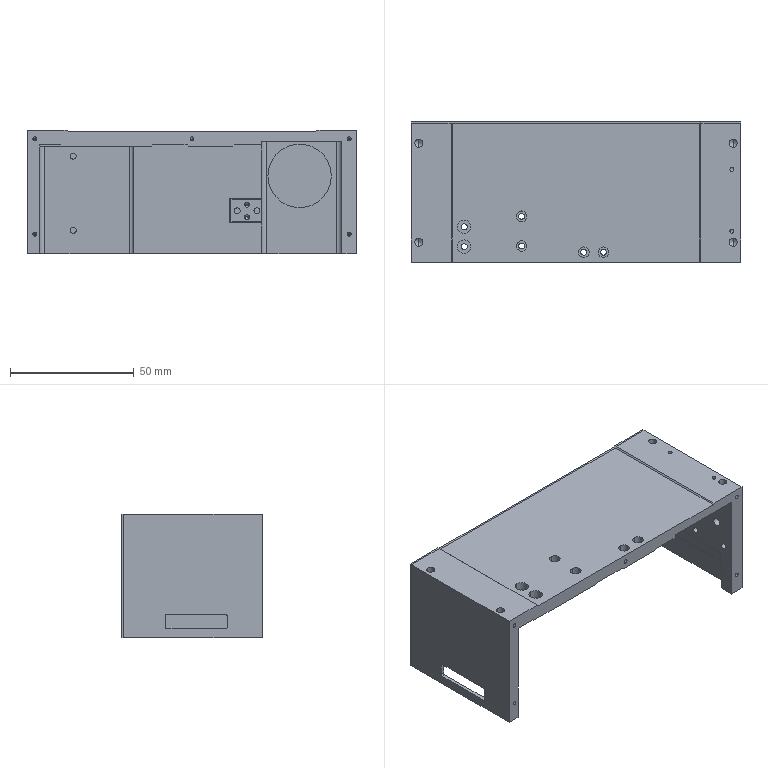NC program | NX | posted with a generic post | part box 133 x 56.74 x 50 mm
Whole program:
N10 G17 G21 G94 G90
(DRILLING_COPY_1 , TOOL : D6A45)
N12 T07 M6
N14 G54
N16 G17 G0 G90 X19.13 Y-28.5 B0. C0. S5000 M3
N18 G43 Z30. H7
N20 G94 G81 G98 Z-1. F250. R3.
N22 X13.13 Y-18.5
N24 X9.13 Y-8.5
N26 X5.13 Y-18.5
N28 X-0.87 Y-28.5
N30 X-7.87
N32 X-11.87 Y-18.5
N34 X-15.87 Y-8.5
N36 X-19.87 Y-18.5
N38 X-23.87 Y-28.5
N40 G80
N42 G0 X-23.87 Y-28.5 Z30.
N44 M5
(DRILLING_COPY_COPY_COPY_COPY , TOOL : 2.5ZT)
N46 T08 M6
N48 G54
N50 G17 G0 G90 X-15.87 Y-8.5 B0. C0. S2000 M3
N52 G43 Z30. H8
N54 G94 G83 G98 Z-8.251 F150. Q2. R3.
N56 X-23.87 Y-28.5
N58 X-7.87
N60 X9.13 Y-8.5
N62 X-0.87 Y-28.5
N64 X19.13
N66 G80
N68 G0 X19.13 Y-28.5 Z30.
N70 M5
(DRILLING_COPY_COPY_COPY_COPY_COPY , TOOL : 3.4ZT)
N72 T02 M6
N74 G54
N76 G17 G0 G90 X-19.87 Y-18.5 B0. C0. S2000 M3
N78 G43 Z30. H2
N80 G94 G83 G98 Z-8.521 F150. Q2. R-0.4
N82 X-11.87
N84 X5.13
N86 X13.13
N88 G80
N90 G0 X13.13 Y-18.5 Z30.
N92 M5
(HOLE_MILLING_COPY , TOOL : D4)
N94 T04 M6
N96 G54
N98 G17 G0 G90 X-19.87 Y-18.5 B0. C0. S9500 M3
N100 G43 Z30. H4
N102 Z0.5
N104 G94 G3 X-18.995 Y-19.375 R0.875 F1250.
N106 X-18.12 Y-18.5 R0.875
N108 X-18.12 Y-18.5 Z0.25 I-1.75 J0.
N110 X-18.12 Y-18.5 Z0. I-1.75 J0.
N112 X-18.12 Y-18.5 Z-0.25 I-1.75 J0.
N114 X-18.12 Y-18.5 Z-0.5 I-1.75 J0.
N116 X-18.12 Y-18.5 Z-0.75 I-1.75 J0.
N118 X-18.12 Y-18.5 Z-1. I-1.75 J0.
N120 X-18.12 Y-18.5 Z-1.25 I-1.75 J0.
N122 X-18.12 Y-18.5 Z-1.5 I-1.75 J0.
N124 X-18.12 Y-18.5 Z-1.75 I-1.75 J0.
N126 X-18.12 Y-18.5 Z-2. I-1.75 J0.
N128 X-18.12 Y-18.5 Z-2.25 I-1.75 J0.
N130 X-18.12 Y-18.5 Z-2.5 I-1.75 J0.
N132 X-18.12 Y-18.5 Z-2.75 I-1.75 J0.
N134 X-18.12 Y-18.5 Z-3. I-1.75 J0.
N136 X-18.12 Y-18.5 Z-3.25 I-1.75 J0.
N138 X-21.286 Y-19.529 Z-3.4 R-1.75
N140 X-18.841 Y-19.916 R1.75
N142 X-21.286 Y-19.529 R-1.75
N144 X-20.064 Y-19.722 R0.875
N146 X-19.87 Y-18.5 R0.875
N148 G0 Z30.
N150 X-11.87
N152 Z0.5
N154 G3 X-10.995 Y-19.375 R0.875
N156 X-10.12 Y-18.5 R0.875
N158 X-10.12 Y-18.5 Z0.25 I-1.75 J0.
N160 X-10.12 Y-18.5 Z0. I-1.75 J0.
N162 X-10.12 Y-18.5 Z-0.25 I-1.75 J0.
N164 X-10.12 Y-18.5 Z-0.5 I-1.75 J0.
N166 X-10.12 Y-18.5 Z-0.75 I-1.75 J0.
N168 X-10.12 Y-18.5 Z-1. I-1.75 J0.
N170 X-10.12 Y-18.5 Z-1.25 I-1.75 J0.
N172 X-10.12 Y-18.5 Z-1.5 I-1.75 J0.
N174 X-10.12 Y-18.5 Z-1.75 I-1.75 J0.
N176 X-10.12 Y-18.5 Z-2. I-1.75 J0.
N178 X-10.12 Y-18.5 Z-2.25 I-1.75 J0.
N180 X-10.12 Y-18.5 Z-2.5 I-1.75 J0.
N182 X-10.12 Y-18.5 Z-2.75 I-1.75 J0.
N184 X-10.12 Y-18.5 Z-3. I-1.75 J0.
N186 X-10.12 Y-18.5 Z-3.25 I-1.75 J0.
N188 X-13.286 Y-19.529 Z-3.4 R-1.75
N190 X-10.841 Y-19.916 R1.75
N192 X-13.286 Y-19.529 R-1.75
N194 X-12.064 Y-19.722 R0.875
N196 X-11.87 Y-18.5 R0.875
N198 G0 Z30.
N200 X5.13
N202 Z0.5
N204 G3 X6.005 Y-19.375 R0.875
N206 X6.88 Y-18.5 R0.875
N208 X6.88 Y-18.5 Z0.25 I-1.75 J0.
N210 X6.88 Y-18.5 Z0. I-1.75 J0.
N212 X6.88 Y-18.5 Z-0.25 I-1.75 J0.
N214 X6.88 Y-18.5 Z-0.5 I-1.75 J0.
N216 X6.88 Y-18.5 Z-0.75 I-1.75 J0.
N218 X6.88 Y-18.5 Z-1. I-1.75 J0.
N220 X6.88 Y-18.5 Z-1.25 I-1.75 J0.
N222 X6.88 Y-18.5 Z-1.5 I-1.75 J0.
N224 X6.88 Y-18.5 Z-1.75 I-1.75 J0.
N226 X6.88 Y-18.5 Z-2. I-1.75 J0.
N228 X6.88 Y-18.5 Z-2.25 I-1.75 J0.
N230 X6.88 Y-18.5 Z-2.5 I-1.75 J0.
N232 X6.88 Y-18.5 Z-2.75 I-1.75 J0.
N234 X6.88 Y-18.5 Z-3. I-1.75 J0.
N236 X6.88 Y-18.5 Z-3.25 I-1.75 J0.
N238 X3.714 Y-19.529 Z-3.4 R-1.75
N240 X6.159 Y-19.916 R1.75
N242 X3.714 Y-19.529 R-1.75
N244 X4.936 Y-19.722 R0.875
N246 X5.13 Y-18.5 R0.875
N248 G0 Z30.
N250 X13.13
N252 Z0.5
N254 G3 X14.005 Y-19.375 R0.875
N256 X14.88 Y-18.5 R0.875
N258 X14.88 Y-18.5 Z0.25 I-1.75 J0.
N260 X14.88 Y-18.5 Z0. I-1.75 J0.
N262 X14.88 Y-18.5 Z-0.25 I-1.75 J0.
N264 X14.88 Y-18.5 Z-0.5 I-1.75 J0.
N266 X14.88 Y-18.5 Z-0.75 I-1.75 J0.
N268 X14.88 Y-18.5 Z-1. I-1.75 J0.
N270 X14.88 Y-18.5 Z-1.25 I-1.75 J0.
N272 X14.88 Y-18.5 Z-1.5 I-1.75 J0.
N274 X14.88 Y-18.5 Z-1.75 I-1.75 J0.
N276 X14.88 Y-18.5 Z-2. I-1.75 J0.
N278 X14.88 Y-18.5 Z-2.25 I-1.75 J0.
N280 X14.88 Y-18.5 Z-2.5 I-1.75 J0.
N282 X14.88 Y-18.5 Z-2.75 I-1.75 J0.
N284 X14.88 Y-18.5 Z-3. I-1.75 J0.
N286 X14.88 Y-18.5 Z-3.25 I-1.75 J0.
N288 X11.714 Y-19.529 Z-3.4 R-1.75
N290 X14.159 Y-19.916 R1.75
N292 X11.714 Y-19.529 R-1.75
N294 X12.936 Y-19.722 R0.875
N296 X13.13 Y-18.5 R0.875
N298 G0 Z30.
N300 M5
(PLANAR_MILL_COPY_1_COPY_COPY , TOOL : D6A45)
N302 T07 M6
N304 G54
N306 G17 G0 G90 X19.43 Y-28.302 B0. C0. S9500 M3
N308 G43 Z30. H7
N310 Z0.5
N312 G94 G1 X19.278 Y-28.15 Z0.442 F1250.
N314 X18.982 Z0.363
N316 X18.78 Y-28.352 Z0.287
N318 Y-28.648 Z0.207
N320 X18.982 Y-28.85 Z0.131
N322 X19.278 Z0.051
N324 X19.48 Y-28.648 Z-0.025
N326 Y-28.352 Z-0.105
N328 X19.278 Y-28.15 Z-0.181
N330 X18.982 Z-0.26
N332 X18.78 Y-28.352 Z-0.337
N334 Y-28.648 Z-0.416
N336 X18.982 Y-28.85 Z-0.493
N338 X19.278 Z-0.572
N340 X19.48 Y-28.648 Z-0.649
N342 Y-28.352 Z-0.728
N344 X19.278 Y-28.15 Z-0.804
N346 X18.982 Z-0.884
N348 X18.78 Y-28.352 Z-0.96
N350 Y-28.5 Z-1.
N352 G3 X19.13 Y-28.85 R0.35
N354 X18.78 Y-28.5 R-0.35
N356 X19.23 Y-28.283 R0.5
N358 G1 Z0.5
N360 G0 Z30.
N362 X11.582 Y-17.929
N364 Z0.5
N366 G1 Z-1.
N368 X10.78 Y-17.634
N370 G3 X10.28 Y-18.5 R1.
N372 X13.13 Y-21.35 R2.85
N374 X10.28 Y-18.5 R-2.85
N376 X10.78 Y-19.366 R1.
N378 G1 X11.582 Y-19.071
N380 Z0.5
N382 G0 Z30.
N384 X9.43 Y-8.302
N386 Z0.5
N388 G1 X9.278 Y-8.15 Z0.442
N390 X8.982 Z0.363
N392 X8.78 Y-8.352 Z0.287
N394 Y-8.648 Z0.207
N396 X8.982 Y-8.85 Z0.131
N398 X9.278 Z0.051
N400 X9.48 Y-8.648 Z-0.025
N402 Y-8.352 Z-0.105
N404 X9.278 Y-8.15 Z-0.181
N406 X8.982 Z-0.26
N408 X8.78 Y-8.352 Z-0.337
N410 Y-8.648 Z-0.416
N412 X8.982 Y-8.85 Z-0.493
N414 X9.278 Z-0.572
N416 X9.48 Y-8.648 Z-0.649
N418 Y-8.352 Z-0.728
N420 X9.278 Y-8.15 Z-0.804
N422 X8.982 Z-0.884
N424 X8.78 Y-8.352 Z-0.96
N426 Y-8.5 Z-1.
N428 G3 X9.13 Y-8.85 R0.35
N430 X8.78 Y-8.5 R-0.35
N432 X9.23 Y-8.283 R0.5
N434 G1 Z0.5
N436 G0 Z30.
N438 X3.582 Y-17.929
N440 Z0.5
N442 G1 Z-1.
N444 X2.78 Y-17.634
N446 G3 X2.28 Y-18.5 R1.
N448 X5.13 Y-21.35 R2.85
N450 X2.28 Y-18.5 R-2.85
N452 X2.78 Y-19.366 R1.
N454 G1 X3.582 Y-19.071
N456 Z0.5
N458 G0 Z30.
N460 X-0.57 Y-28.302
N462 Z0.5
N464 G1 X-0.722 Y-28.15 Z0.442
N466 X-1.018 Z0.363
N468 X-1.22 Y-28.352 Z0.287
N470 Y-28.648 Z0.207
N472 X-1.018 Y-28.85 Z0.131
N474 X-0.722 Z0.051
N476 X-0.52 Y-28.648 Z-0.025
N478 Y-28.352 Z-0.105
N480 X-0.722 Y-28.15 Z-0.181
N482 X-1.018 Z-0.26
N484 X-1.22 Y-28.352 Z-0.337
N486 Y-28.648 Z-0.416
N488 X-1.018 Y-28.85 Z-0.493
N490 X-0.722 Z-0.572
N492 X-0.52 Y-28.648 Z-0.649
N494 Y-28.352 Z-0.728
N496 X-0.722 Y-28.15 Z-0.804
N498 X-1.018 Z-0.884
N500 X-1.22 Y-28.352 Z-0.96
N502 Y-28.5 Z-1.
N504 G3 X-0.87 Y-28.85 R0.35
N506 X-1.22 Y-28.5 R-0.35
N508 X-0.77 Y-28.283 R0.5
N510 G1 Z0.5
N512 G0 Z30.
N514 X-7.57 Y-28.302
N516 Z0.5
N518 G1 X-7.722 Y-28.15 Z0.442
N520 X-8.018 Z0.363
N522 X-8.22 Y-28.352 Z0.287
N524 Y-28.648 Z0.207
N526 X-8.018 Y-28.85 Z0.131
N528 X-7.722 Z0.051
N530 X-7.52 Y-28.648 Z-0.025
N532 Y-28.352 Z-0.105
N534 X-7.722 Y-28.15 Z-0.181
N536 X-8.018 Z-0.26
N538 X-8.22 Y-28.352 Z-0.337
N540 Y-28.648 Z-0.416
N542 X-8.018 Y-28.85 Z-0.493
N544 X-7.722 Z-0.572
N546 X-7.52 Y-28.648 Z-0.649
N548 Y-28.352 Z-0.728
N550 X-7.722 Y-28.15 Z-0.804
N552 X-8.018 Z-0.884
N554 X-8.22 Y-28.352 Z-0.96
N556 Y-28.5 Z-1.
N558 G3 X-7.87 Y-28.85 R0.35
N560 X-8.22 Y-28.5 R-0.35
N562 X-7.77 Y-28.283 R0.5
N564 G1 Z0.5
N566 G0 Z30.
N568 X-13.418 Y-17.929
N570 Z0.5
N572 G1 Z-1.
N574 X-14.22 Y-17.634
N576 G3 X-14.72 Y-18.5 R1.
N578 X-11.87 Y-21.35 R2.85
N580 X-14.72 Y-18.5 R-2.85
N582 X-14.22 Y-19.366 R1.
N584 G1 X-13.418 Y-19.071
N586 Z0.5
N588 G0 Z30.
N590 X-15.57 Y-8.302
N592 Z0.5
N594 G1 X-15.722 Y-8.15 Z0.442
N596 X-16.018 Z0.363
N598 X-16.22 Y-8.352 Z0.287
N600 Y-8.648 Z0.207
N602 X-16.018 Y-8.85 Z0.131
N604 X-15.722 Z0.051
N606 X-15.52 Y-8.648 Z-0.025
N608 Y-8.352 Z-0.105
N610 X-15.722 Y-8.15 Z-0.181
N612 X-16.018 Z-0.26
N614 X-16.22 Y-8.352 Z-0.337
N616 Y-8.648 Z-0.416
N618 X-16.018 Y-8.85 Z-0.493
N620 X-15.722 Z-0.572
N622 X-15.52 Y-8.648 Z-0.649
N624 Y-8.352 Z-0.728
N626 X-15.722 Y-8.15 Z-0.804
N628 X-16.018 Z-0.884
N630 X-16.22 Y-8.352 Z-0.96
N632 Y-8.5 Z-1.
N634 G3 X-15.87 Y-8.85 R0.35
N636 X-16.22 Y-8.5 R-0.35
N638 X-15.77 Y-8.283 R0.5
N640 G1 Z0.5
N642 G0 Z30.
N644 X-21.418 Y-17.929
N646 Z0.5
N648 G1 Z-1.
N650 X-22.22 Y-17.634
N652 G3 X-22.72 Y-18.5 R1.
N654 X-19.87 Y-21.35 R2.85
N656 X-22.72 Y-18.5 R-2.85
N658 X-22.22 Y-19.366 R1.
N660 G1 X-21.418 Y-19.071
N662 Z0.5
N664 G0 Z30.
N666 X-23.57 Y-28.302
N668 Z0.5
N670 G1 X-23.722 Y-28.15 Z0.442
N672 X-24.018 Z0.363
N674 X-24.22 Y-28.352 Z0.287
N676 Y-28.648 Z0.207
N678 X-24.018 Y-28.85 Z0.131
N680 X-23.722 Z0.051
N682 X-23.52 Y-28.648 Z-0.025
N684 Y-28.352 Z-0.105
N686 X-23.722 Y-28.15 Z-0.181
N688 X-24.018 Z-0.26
N690 X-24.22 Y-28.352 Z-0.337
N692 Y-28.648 Z-0.416
N694 X-24.018 Y-28.85 Z-0.493
N696 X-23.722 Z-0.572
N698 X-23.52 Y-28.648 Z-0.649
N700 Y-28.352 Z-0.728
N702 X-23.722 Y-28.15 Z-0.804
N704 X-24.018 Z-0.884
N706 X-24.22 Y-28.352 Z-0.96
N708 Y-28.5 Z-1.
N710 G3 X-23.87 Y-28.85 R0.35
N712 X-24.22 Y-28.5 R-0.35
N714 X-23.77 Y-28.283 R0.5
N716 G1 Z0.5
N718 G0 Z30.
N720 M5
N722 M2